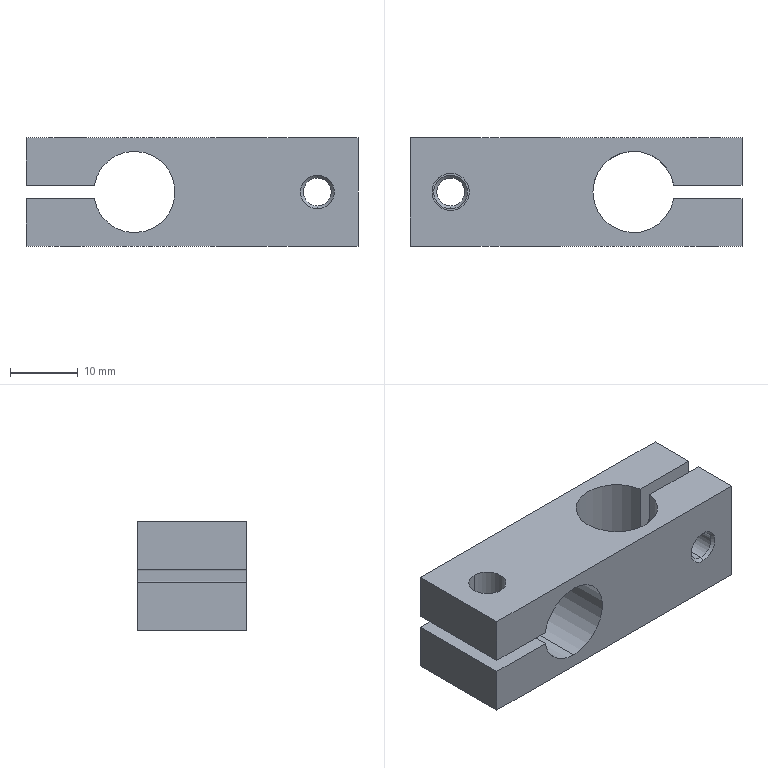Part | STEP file | 11-KDST12_b-ab11 | 1 solid | 33 faces | box 49 x 16 x 16 mm | volume 7757 mm3 | cylinder 13 | plane 12 | cone 8 | commonest cylinder face diameters 12 x5 4.134 x4 5.5 x4
STEP:
#1=CARTESIAN_POINT('',(-27.,2.75,1.));
#2=VERTEX_POINT('',#1);
#3=CARTESIAN_POINT('',(-27.,-2.75,1.));
#4=VERTEX_POINT('',#3);
#5=CARTESIAN_POINT('',(-27.,0.,1.));
#6=DIRECTION('',(0.,0.,1.));
#7=DIRECTION('',(-1.,0.,0.));
#8=AXIS2_PLACEMENT_3D('',#5,#6,#7);
#9=CIRCLE('',#8,2.75);
#10=EDGE_CURVE('',#2,#4,#9,.T.);
#11=ORIENTED_EDGE('',*,*,#10,.F.);
#12=CARTESIAN_POINT('',(-27.,2.75,8.));
#13=VERTEX_POINT('',#12);
#14=CARTESIAN_POINT('',(-27.,2.75,-8.));
#15=DIRECTION('',(0.,0.,1.));
#16=VECTOR('',#15,1000.);
#17=LINE('',#14,#16);
#18=EDGE_CURVE('',#2,#13,#17,.T.);
#19=ORIENTED_EDGE('',*,*,#18,.T.);
#20=CARTESIAN_POINT('',(-27.,-2.75,8.));
#21=VERTEX_POINT('',#20);
#22=CARTESIAN_POINT('',(-27.,0.,8.));
#23=DIRECTION('',(0.,0.,1.));
#24=DIRECTION('',(0.,-1.,0.));
#25=AXIS2_PLACEMENT_3D('',#22,#23,#24);
#26=CIRCLE('',#25,2.75);
#27=EDGE_CURVE('',#13,#21,#26,.T.);
#28=ORIENTED_EDGE('',*,*,#27,.T.);
#29=CARTESIAN_POINT('',(-27.,-2.75,-8.));
#30=DIRECTION('',(0.,0.,1.));
#31=VECTOR('',#30,1000.);
#32=LINE('',#29,#31);
#33=EDGE_CURVE('',#4,#21,#32,.T.);
#34=ORIENTED_EDGE('',*,*,#33,.F.);
#35=EDGE_LOOP('',(#11,#19,#28,#34));
#36=FACE_OUTER_BOUND('',#35,.T.);
#37=CARTESIAN_POINT('',(-27.,0.,-8.));
#38=DIRECTION('',(0.,0.,1.));
#39=DIRECTION('',(0.,-1.,0.));
#40=AXIS2_PLACEMENT_3D('',#37,#38,#39);
#41=CYLINDRICAL_SURFACE('',#40,2.75);
#42=ADVANCED_FACE('',(#36),#41,.F.);
#43=CARTESIAN_POINT('',(-27.,2.067,-1.433));
#44=VERTEX_POINT('',#43);
#45=CARTESIAN_POINT('',(-27.,-2.067,-1.433));
#46=VERTEX_POINT('',#45);
#47=CARTESIAN_POINT('',(-27.,0.,-1.433));
#48=DIRECTION('',(0.,0.,1.));
#49=DIRECTION('',(0.,-1.,0.));
#50=AXIS2_PLACEMENT_3D('',#47,#48,#49);
#51=CIRCLE('',#50,2.067);
#52=EDGE_CURVE('',#44,#46,#51,.T.);
#53=ORIENTED_EDGE('',*,*,#52,.F.);
#54=CARTESIAN_POINT('',(-27.,2.5,-1.));
#55=VERTEX_POINT('',#54);
#56=CARTESIAN_POINT('',(-27.,2.067,-1.433));
#57=DIRECTION('',(0.,0.7071,0.7071));
#58=VECTOR('',#57,1000.);
#59=LINE('',#56,#58);
#60=EDGE_CURVE('',#44,#55,#59,.T.);
#61=ORIENTED_EDGE('',*,*,#60,.T.);
#62=CARTESIAN_POINT('',(-27.,-2.5,-1.));
#63=VERTEX_POINT('',#62);
#64=CARTESIAN_POINT('',(-27.,0.,-1.));
#65=DIRECTION('',(0.,0.,1.));
#66=DIRECTION('',(0.,-1.,0.));
#67=AXIS2_PLACEMENT_3D('',#64,#65,#66);
#68=CIRCLE('',#67,2.5);
#69=EDGE_CURVE('',#55,#63,#68,.T.);
#70=ORIENTED_EDGE('',*,*,#69,.T.);
#71=CARTESIAN_POINT('',(-27.,-2.067,-1.433));
#72=DIRECTION('',(0.,-0.7071,0.7071));
#73=VECTOR('',#72,1000.);
#74=LINE('',#71,#73);
#75=EDGE_CURVE('',#46,#63,#74,.T.);
#76=ORIENTED_EDGE('',*,*,#75,.F.);
#77=EDGE_LOOP('',(#53,#61,#70,#76));
#78=FACE_OUTER_BOUND('',#77,.T.);
#79=CARTESIAN_POINT('',(-27.,0.,-1.433));
#80=DIRECTION('',(0.,0.,1.));
#81=DIRECTION('',(0.,-1.,0.));
#82=AXIS2_PLACEMENT_3D('',#79,#80,#81);
#83=CONICAL_SURFACE('',#82,2.067,0.7854);
#84=ADVANCED_FACE('',(#78),#83,.F.);
#85=CARTESIAN_POINT('',(-27.,2.067,-7.567));
#86=VERTEX_POINT('',#85);
#87=CARTESIAN_POINT('',(-27.,-2.067,-7.567));
#88=VERTEX_POINT('',#87);
#89=CARTESIAN_POINT('',(-27.,0.,-7.567));
#90=DIRECTION('',(0.,0.,1.));
#91=DIRECTION('',(0.,-1.,0.));
#92=AXIS2_PLACEMENT_3D('',#89,#90,#91);
#93=CIRCLE('',#92,2.067);
#94=EDGE_CURVE('',#86,#88,#93,.T.);
#95=ORIENTED_EDGE('',*,*,#94,.F.);
#96=CARTESIAN_POINT('',(-27.,2.067,-8.));
#97=DIRECTION('',(0.,0.,1.));
#98=VECTOR('',#97,1000.);
#99=LINE('',#96,#98);
#100=EDGE_CURVE('',#86,#44,#99,.T.);
#101=ORIENTED_EDGE('',*,*,#100,.T.);
#102=ORIENTED_EDGE('',*,*,#52,.T.);
#103=CARTESIAN_POINT('',(-27.,-2.067,-8.));
#104=DIRECTION('',(0.,0.,1.));
#105=VECTOR('',#104,1000.);
#106=LINE('',#103,#105);
#107=EDGE_CURVE('',#88,#46,#106,.T.);
#108=ORIENTED_EDGE('',*,*,#107,.F.);
#109=EDGE_LOOP('',(#95,#101,#102,#108));
#110=FACE_OUTER_BOUND('',#109,.T.);
#111=CARTESIAN_POINT('',(-27.,0.,-8.));
#112=DIRECTION('',(0.,0.,1.));
#113=DIRECTION('',(0.,-1.,0.));
#114=AXIS2_PLACEMENT_3D('',#111,#112,#113);
#115=CYLINDRICAL_SURFACE('',#114,2.067);
#116=ADVANCED_FACE('',(#110),#115,.F.);
#117=ORIENTED_EDGE('',*,*,#94,.T.);
#118=CARTESIAN_POINT('',(-27.,-2.5,-8.));
#119=VERTEX_POINT('',#118);
#120=CARTESIAN_POINT('',(-27.,-2.5,-8.));
#121=DIRECTION('',(0.,-0.7071,-0.7071));
#122=VECTOR('',#121,1000.);
#123=LINE('',#120,#122);
#124=EDGE_CURVE('',#88,#119,#123,.T.);
#125=ORIENTED_EDGE('',*,*,#124,.T.);
#126=CARTESIAN_POINT('',(-27.,2.5,-8.));
#127=VERTEX_POINT('',#126);
#128=CARTESIAN_POINT('',(-27.,0.,-8.));
#129=DIRECTION('',(0.,0.,1.));
#130=DIRECTION('',(0.,-1.,0.));
#131=AXIS2_PLACEMENT_3D('',#128,#129,#130);
#132=CIRCLE('',#131,2.5);
#133=EDGE_CURVE('',#127,#119,#132,.T.);
#134=ORIENTED_EDGE('',*,*,#133,.F.);
#135=CARTESIAN_POINT('',(-27.,2.5,-8.));
#136=DIRECTION('',(0.,0.7071,-0.7071));
#137=VECTOR('',#136,1000.);
#138=LINE('',#135,#137);
#139=EDGE_CURVE('',#86,#127,#138,.T.);
#140=ORIENTED_EDGE('',*,*,#139,.F.);
#141=EDGE_LOOP('',(#117,#125,#134,#140));
#142=FACE_OUTER_BOUND('',#141,.T.);
#143=CARTESIAN_POINT('',(-27.,0.,-8.));
#144=DIRECTION('',(0.,0.,-1.));
#145=DIRECTION('',(0.,1.,0.));
#146=AXIS2_PLACEMENT_3D('',#143,#144,#145);
#147=CONICAL_SURFACE('',#146,2.5,0.7854);
#148=ADVANCED_FACE('',(#142),#147,.F.);
#149=CARTESIAN_POINT('',(10.,-7.567,-2.067));
#150=VERTEX_POINT('',#149);
#151=CARTESIAN_POINT('',(10.,-7.567,2.067));
#152=VERTEX_POINT('',#151);
#153=CARTESIAN_POINT('',(10.,-7.567,0.));
#154=DIRECTION('',(0.,1.,0.));
#155=DIRECTION('',(0.,0.,1.));
#156=AXIS2_PLACEMENT_3D('',#153,#154,#155);
#157=CIRCLE('',#156,2.067);
#158=EDGE_CURVE('',#150,#152,#157,.T.);
#159=ORIENTED_EDGE('',*,*,#158,.T.);
#160=CARTESIAN_POINT('',(10.,-8.,2.5));
#161=VERTEX_POINT('',#160);
#162=CARTESIAN_POINT('',(10.,-8.,2.5));
#163=DIRECTION('',(0.,-0.7071,0.7071));
#164=VECTOR('',#163,1000.);
#165=LINE('',#162,#164);
#166=EDGE_CURVE('',#152,#161,#165,.T.);
#167=ORIENTED_EDGE('',*,*,#166,.T.);
#168=CARTESIAN_POINT('',(10.,-8.,-2.5));
#169=VERTEX_POINT('',#168);
#170=CARTESIAN_POINT('',(10.,-8.,0.));
#171=DIRECTION('',(0.,1.,0.));
#172=DIRECTION('',(0.,0.,1.));
#173=AXIS2_PLACEMENT_3D('',#170,#171,#172);
#174=CIRCLE('',#173,2.5);
#175=EDGE_CURVE('',#169,#161,#174,.T.);
#176=ORIENTED_EDGE('',*,*,#175,.F.);
#177=CARTESIAN_POINT('',(10.,-8.,-2.5));
#178=DIRECTION('',(0.,-0.7071,-0.7071));
#179=VECTOR('',#178,1000.);
#180=LINE('',#177,#179);
#181=EDGE_CURVE('',#150,#169,#180,.T.);
#182=ORIENTED_EDGE('',*,*,#181,.F.);
#183=EDGE_LOOP('',(#159,#167,#176,#182));
#184=FACE_OUTER_BOUND('',#183,.T.);
#185=CARTESIAN_POINT('',(10.,-8.,0.));
#186=DIRECTION('',(0.,-1.,0.));
#187=DIRECTION('',(0.,0.,-1.));
#188=AXIS2_PLACEMENT_3D('',#185,#186,#187);
#189=CONICAL_SURFACE('',#188,2.5,0.7854);
#190=ADVANCED_FACE('',(#184),#189,.F.);
#191=ORIENTED_EDGE('',*,*,#158,.F.);
#192=CARTESIAN_POINT('',(10.,-1.433,-2.067));
#193=VERTEX_POINT('',#192);
#194=CARTESIAN_POINT('',(10.,-8.,-2.067));
#195=DIRECTION('',(0.,1.,0.));
#196=VECTOR('',#195,1000.);
#197=LINE('',#194,#196);
#198=EDGE_CURVE('',#150,#193,#197,.T.);
#199=ORIENTED_EDGE('',*,*,#198,.T.);
#200=CARTESIAN_POINT('',(10.,-1.433,2.067));
#201=VERTEX_POINT('',#200);
#202=CARTESIAN_POINT('',(10.,-1.433,0.));
#203=DIRECTION('',(0.,1.,0.));
#204=DIRECTION('',(0.,0.,1.));
#205=AXIS2_PLACEMENT_3D('',#202,#203,#204);
#206=CIRCLE('',#205,2.067);
#207=EDGE_CURVE('',#193,#201,#206,.T.);
#208=ORIENTED_EDGE('',*,*,#207,.T.);
#209=CARTESIAN_POINT('',(10.,-8.,2.067));
#210=DIRECTION('',(0.,1.,0.));
#211=VECTOR('',#210,1000.);
#212=LINE('',#209,#211);
#213=EDGE_CURVE('',#152,#201,#212,.T.);
#214=ORIENTED_EDGE('',*,*,#213,.F.);
#215=EDGE_LOOP('',(#191,#199,#208,#214));
#216=FACE_OUTER_BOUND('',#215,.T.);
#217=CARTESIAN_POINT('',(10.,-8.,0.));
#218=DIRECTION('',(0.,1.,0.));
#219=DIRECTION('',(0.,0.,1.));
#220=AXIS2_PLACEMENT_3D('',#217,#218,#219);
#221=CYLINDRICAL_SURFACE('',#220,2.067);
#222=ADVANCED_FACE('',(#216),#221,.F.);
#223=ORIENTED_EDGE('',*,*,#207,.F.);
#224=CARTESIAN_POINT('',(10.,-1.,-2.5));
#225=VERTEX_POINT('',#224);
#226=CARTESIAN_POINT('',(10.,-1.433,-2.067));
#227=DIRECTION('',(0.,0.7071,-0.7071));
#228=VECTOR('',#227,1000.);
#229=LINE('',#226,#228);
#230=EDGE_CURVE('',#193,#225,#229,.T.);
#231=ORIENTED_EDGE('',*,*,#230,.T.);
#232=CARTESIAN_POINT('',(10.,-1.,2.5));
#233=VERTEX_POINT('',#232);
#234=CARTESIAN_POINT('',(10.,-1.,0.));
#235=DIRECTION('',(0.,1.,0.));
#236=DIRECTION('',(0.,0.,1.));
#237=AXIS2_PLACEMENT_3D('',#234,#235,#236);
#238=CIRCLE('',#237,2.5);
#239=EDGE_CURVE('',#225,#233,#238,.T.);
#240=ORIENTED_EDGE('',*,*,#239,.T.);
#241=CARTESIAN_POINT('',(10.,-1.433,2.067));
#242=DIRECTION('',(0.,0.7071,0.7071));
#243=VECTOR('',#242,1000.);
#244=LINE('',#241,#243);
#245=EDGE_CURVE('',#201,#233,#244,.T.);
#246=ORIENTED_EDGE('',*,*,#245,.F.);
#247=EDGE_LOOP('',(#223,#231,#240,#246));
#248=FACE_OUTER_BOUND('',#247,.T.);
#249=CARTESIAN_POINT('',(10.,-1.433,0.));
#250=DIRECTION('',(0.,1.,0.));
#251=DIRECTION('',(0.,0.,1.));
#252=AXIS2_PLACEMENT_3D('',#249,#250,#251);
#253=CONICAL_SURFACE('',#252,2.067,0.7854);
#254=ADVANCED_FACE('',(#248),#253,.F.);
#255=CARTESIAN_POINT('',(10.,1.,2.75));
#256=VERTEX_POINT('',#255);
#257=CARTESIAN_POINT('',(10.,1.,-2.75));
#258=VERTEX_POINT('',#257);
#259=CARTESIAN_POINT('',(10.,1.,0.));
#260=DIRECTION('',(0.,-1.,0.));
#261=DIRECTION('',(0.,0.,1.));
#262=AXIS2_PLACEMENT_3D('',#259,#260,#261);
#263=CIRCLE('',#262,2.75);
#264=EDGE_CURVE('',#256,#258,#263,.T.);
#265=ORIENTED_EDGE('',*,*,#264,.T.);
#266=CARTESIAN_POINT('',(10.,8.,-2.75));
#267=VERTEX_POINT('',#266);
#268=CARTESIAN_POINT('',(10.,-8.,-2.75));
#269=DIRECTION('',(0.,1.,0.));
#270=VECTOR('',#269,1000.);
#271=LINE('',#268,#270);
#272=EDGE_CURVE('',#258,#267,#271,.T.);
#273=ORIENTED_EDGE('',*,*,#272,.T.);
#274=CARTESIAN_POINT('',(10.,8.,2.75));
#275=VERTEX_POINT('',#274);
#276=CARTESIAN_POINT('',(10.,8.,0.));
#277=DIRECTION('',(0.,1.,0.));
#278=DIRECTION('',(0.,0.,1.));
#279=AXIS2_PLACEMENT_3D('',#276,#277,#278);
#280=CIRCLE('',#279,2.75);
#281=EDGE_CURVE('',#267,#275,#280,.T.);
#282=ORIENTED_EDGE('',*,*,#281,.T.);
#283=CARTESIAN_POINT('',(10.,-8.,2.75));
#284=DIRECTION('',(0.,1.,0.));
#285=VECTOR('',#284,1000.);
#286=LINE('',#283,#285);
#287=EDGE_CURVE('',#256,#275,#286,.T.);
#288=ORIENTED_EDGE('',*,*,#287,.F.);
#289=EDGE_LOOP('',(#265,#273,#282,#288));
#290=FACE_OUTER_BOUND('',#289,.T.);
#291=CARTESIAN_POINT('',(10.,-8.,0.));
#292=DIRECTION('',(0.,1.,0.));
#293=DIRECTION('',(0.,0.,1.));
#294=AXIS2_PLACEMENT_3D('',#291,#292,#293);
#295=CYLINDRICAL_SURFACE('',#294,2.75);
#296=ADVANCED_FACE('',(#290),#295,.F.);
#297=CARTESIAN_POINT('',(-22.916,-8.,-1.));
#298=VERTEX_POINT('',#297);
#299=CARTESIAN_POINT('',(-17.,-8.,-6.));
#300=VERTEX_POINT('',#299);
#301=CARTESIAN_POINT('',(-17.,-8.,0.));
#302=DIRECTION('',(0.,-1.,0.));
#303=DIRECTION('',(0.,0.,-1.));
#304=AXIS2_PLACEMENT_3D('',#301,#302,#303);
#305=CIRCLE('',#304,6.);
#306=EDGE_CURVE('',#298,#300,#305,.T.);
#307=ORIENTED_EDGE('',*,*,#306,.T.);
#308=CARTESIAN_POINT('',(-17.,8.,-6.));
#309=VERTEX_POINT('',#308);
#310=CARTESIAN_POINT('',(-17.,-8.,-6.));
#311=DIRECTION('',(0.,1.,0.));
#312=VECTOR('',#311,1000.);
#313=LINE('',#310,#312);
#314=EDGE_CURVE('',#300,#309,#313,.T.);
#315=ORIENTED_EDGE('',*,*,#314,.T.);
#316=CARTESIAN_POINT('',(-22.916,8.,-1.));
#317=VERTEX_POINT('',#316);
#318=CARTESIAN_POINT('',(-17.,8.,0.));
#319=DIRECTION('',(0.,-1.,0.));
#320=DIRECTION('',(0.,0.,-1.));
#321=AXIS2_PLACEMENT_3D('',#318,#319,#320);
#322=CIRCLE('',#321,6.);
#323=EDGE_CURVE('',#317,#309,#322,.T.);
#324=ORIENTED_EDGE('',*,*,#323,.F.);
#325=CARTESIAN_POINT('',(-22.916,-8.,-1.));
#326=DIRECTION('',(0.,1.,0.));
#327=VECTOR('',#326,1000.);
#328=LINE('',#325,#327);
#329=EDGE_CURVE('',#298,#317,#328,.T.);
#330=ORIENTED_EDGE('',*,*,#329,.F.);
#331=EDGE_LOOP('',(#307,#315,#324,#330));
#332=FACE_OUTER_BOUND('',#331,.T.);
#333=CARTESIAN_POINT('',(-17.,-8.,0.));
#334=DIRECTION('',(0.,1.,0.));
#335=DIRECTION('',(0.,0.,1.));
#336=AXIS2_PLACEMENT_3D('',#333,#334,#335);
#337=CYLINDRICAL_SURFACE('',#336,6.);
#338=ADVANCED_FACE('',(#332),#337,.F.);
#339=ORIENTED_EDGE('',*,*,#314,.F.);
#340=CARTESIAN_POINT('',(-17.,-8.,6.));
#341=VERTEX_POINT('',#340);
#342=CARTESIAN_POINT('',(-17.,-8.,0.));
#343=DIRECTION('',(0.,-1.,0.));
#344=DIRECTION('',(0.,0.,-1.));
#345=AXIS2_PLACEMENT_3D('',#342,#343,#344);
#346=CIRCLE('',#345,6.);
#347=EDGE_CURVE('',#300,#341,#346,.T.);
#348=ORIENTED_EDGE('',*,*,#347,.T.);
#349=CARTESIAN_POINT('',(-17.,8.,6.));
#350=VERTEX_POINT('',#349);
#351=CARTESIAN_POINT('',(-17.,-8.,6.));
#352=DIRECTION('',(0.,1.,0.));
#353=VECTOR('',#352,1000.);
#354=LINE('',#351,#353);
#355=EDGE_CURVE('',#341,#350,#354,.T.);
#356=ORIENTED_EDGE('',*,*,#355,.T.);
#357=CARTESIAN_POINT('',(-17.,8.,0.));
#358=DIRECTION('',(0.,-1.,0.));
#359=DIRECTION('',(0.,0.,-1.));
#360=AXIS2_PLACEMENT_3D('',#357,#358,#359);
#361=CIRCLE('',#360,6.);
#362=EDGE_CURVE('',#309,#350,#361,.T.);
#363=ORIENTED_EDGE('',*,*,#362,.F.);
#364=EDGE_LOOP('',(#339,#348,#356,#363));
#365=FACE_OUTER_BOUND('',#364,.T.);
#366=CARTESIAN_POINT('',(-17.,-8.,0.));
#367=DIRECTION('',(0.,1.,0.));
#368=DIRECTION('',(0.,0.,1.));
#369=AXIS2_PLACEMENT_3D('',#366,#367,#368);
#370=CYLINDRICAL_SURFACE('',#369,6.);
#371=ADVANCED_FACE('',(#365),#370,.F.);
#372=CARTESIAN_POINT('',(-6.,0.,8.));
#373=VERTEX_POINT('',#372);
#374=CARTESIAN_POINT('',(5.916,1.,8.));
#375=VERTEX_POINT('',#374);
#376=CARTESIAN_POINT('',(0.,0.,8.));
#377=DIRECTION('',(0.,0.,-1.));
#378=DIRECTION('',(-1.,0.,0.));
#379=AXIS2_PLACEMENT_3D('',#376,#377,#378);
#380=CIRCLE('',#379,6.);
#381=EDGE_CURVE('',#373,#375,#380,.T.);
#382=ORIENTED_EDGE('',*,*,#381,.F.);
#383=CARTESIAN_POINT('',(-6.,0.,-8.));
#384=VERTEX_POINT('',#383);
#385=CARTESIAN_POINT('',(-6.,0.,8.));
#386=DIRECTION('',(0.,0.,-1.));
#387=VECTOR('',#386,1000.);
#388=LINE('',#385,#387);
#389=EDGE_CURVE('',#373,#384,#388,.T.);
#390=ORIENTED_EDGE('',*,*,#389,.T.);
#391=CARTESIAN_POINT('',(5.916,1.,-8.));
#392=VERTEX_POINT('',#391);
#393=CARTESIAN_POINT('',(0.,0.,-8.));
#394=DIRECTION('',(0.,0.,-1.));
#395=DIRECTION('',(-1.,0.,0.));
#396=AXIS2_PLACEMENT_3D('',#393,#394,#395);
#397=CIRCLE('',#396,6.);
#398=EDGE_CURVE('',#384,#392,#397,.T.);
#399=ORIENTED_EDGE('',*,*,#398,.T.);
#400=CARTESIAN_POINT('',(5.916,1.,8.));
#401=DIRECTION('',(0.,0.,-1.));
#402=VECTOR('',#401,1000.);
#403=LINE('',#400,#402);
#404=EDGE_CURVE('',#375,#392,#403,.T.);
#405=ORIENTED_EDGE('',*,*,#404,.F.);
#406=EDGE_LOOP('',(#382,#390,#399,#405));
#407=FACE_OUTER_BOUND('',#406,.T.);
#408=CARTESIAN_POINT('',(0.,0.,8.));
#409=DIRECTION('',(0.,0.,-1.));
#410=DIRECTION('',(-1.,0.,0.));
#411=AXIS2_PLACEMENT_3D('',#408,#409,#410);
#412=CYLINDRICAL_SURFACE('',#411,6.);
#413=ADVANCED_FACE('',(#407),#412,.F.);
#414=CARTESIAN_POINT('',(10.,8.,0.));
#415=DIRECTION('',(0.,1.,0.));
#416=DIRECTION('',(0.,0.,1.));
#417=AXIS2_PLACEMENT_3D('',#414,#415,#416);
#418=CIRCLE('',#417,2.75);
#419=EDGE_CURVE('',#275,#267,#418,.T.);
#420=ORIENTED_EDGE('',*,*,#419,.F.);
#421=ORIENTED_EDGE('',*,*,#281,.F.);
#422=EDGE_LOOP('',(#420,#421));
#423=FACE_BOUND('',#422,.T.);
#424=CARTESIAN_POINT('',(-22.916,8.,1.));
#425=VERTEX_POINT('',#424);
#426=CARTESIAN_POINT('',(-33.,8.,1.));
#427=VERTEX_POINT('',#426);
#428=CARTESIAN_POINT('',(-22.916,8.,1.));
#429=DIRECTION('',(-1.,0.,0.));
#430=VECTOR('',#429,1000.);
#431=LINE('',#428,#430);
#432=EDGE_CURVE('',#425,#427,#431,.T.);
#433=ORIENTED_EDGE('',*,*,#432,.T.);
#434=CARTESIAN_POINT('',(-33.,8.,8.));
#435=VERTEX_POINT('',#434);
#436=CARTESIAN_POINT('',(-33.,8.,8.));
#437=DIRECTION('',(0.,0.,-1.));
#438=VECTOR('',#437,1000.);
#439=LINE('',#436,#438);
#440=EDGE_CURVE('',#435,#427,#439,.T.);
#441=ORIENTED_EDGE('',*,*,#440,.F.);
#442=CARTESIAN_POINT('',(16.,8.,8.));
#443=VERTEX_POINT('',#442);
#444=CARTESIAN_POINT('',(16.,8.,8.));
#445=DIRECTION('',(-1.,0.,0.));
#446=VECTOR('',#445,1000.);
#447=LINE('',#444,#446);
#448=EDGE_CURVE('',#443,#435,#447,.T.);
#449=ORIENTED_EDGE('',*,*,#448,.F.);
#450=CARTESIAN_POINT('',(16.,8.,-8.));
#451=VERTEX_POINT('',#450);
#452=CARTESIAN_POINT('',(16.,8.,8.));
#453=DIRECTION('',(0.,0.,-1.));
#454=VECTOR('',#453,1000.);
#455=LINE('',#452,#454);
#456=EDGE_CURVE('',#443,#451,#455,.T.);
#457=ORIENTED_EDGE('',*,*,#456,.T.);
#458=CARTESIAN_POINT('',(-33.,8.,-8.));
#459=VERTEX_POINT('',#458);
#460=CARTESIAN_POINT('',(16.,8.,-8.));
#461=DIRECTION('',(-1.,0.,0.));
#462=VECTOR('',#461,1000.);
#463=LINE('',#460,#462);
#464=EDGE_CURVE('',#451,#459,#463,.T.);
#465=ORIENTED_EDGE('',*,*,#464,.T.);
#466=CARTESIAN_POINT('',(-33.,8.,-1.));
#467=VERTEX_POINT('',#466);
#468=CARTESIAN_POINT('',(-33.,8.,8.));
#469=DIRECTION('',(0.,0.,-1.));
#470=VECTOR('',#469,1000.);
#471=LINE('',#468,#470);
#472=EDGE_CURVE('',#467,#459,#471,.T.);
#473=ORIENTED_EDGE('',*,*,#472,.F.);
#474=CARTESIAN_POINT('',(-33.,8.,-1.));
#475=DIRECTION('',(1.,0.,0.));
#476=VECTOR('',#475,1000.);
#477=LINE('',#474,#476);
#478=EDGE_CURVE('',#467,#317,#477,.T.);
#479=ORIENTED_EDGE('',*,*,#478,.T.);
#480=ORIENTED_EDGE('',*,*,#323,.T.);
#481=ORIENTED_EDGE('',*,*,#362,.T.);
#482=CARTESIAN_POINT('',(-17.,8.,0.));
#483=DIRECTION('',(0.,-1.,0.));
#484=DIRECTION('',(0.,0.,-1.));
#485=AXIS2_PLACEMENT_3D('',#482,#483,#484);
#486=CIRCLE('',#485,6.);
#487=EDGE_CURVE('',#350,#425,#486,.T.);
#488=ORIENTED_EDGE('',*,*,#487,.T.);
#489=EDGE_LOOP('',(#433,#441,#449,#457,#465,#473,#479,#480,#481,#488));
#490=FACE_OUTER_BOUND('',#489,.T.);
#491=CARTESIAN_POINT('',(16.,8.,8.));
#492=DIRECTION('',(0.,-1.,0.));
#493=DIRECTION('',(0.,0.,-1.));
#494=AXIS2_PLACEMENT_3D('',#491,#492,#493);
#495=PLANE('',#494);
#496=ADVANCED_FACE('',(#423,#490),#495,.F.);
#497=CARTESIAN_POINT('',(-33.,-8.,1.));
#498=VERTEX_POINT('',#497);
#499=CARTESIAN_POINT('',(-33.,-8.,1.));
#500=DIRECTION('',(0.,1.,0.));
#501=VECTOR('',#500,1000.);
#502=LINE('',#499,#501);
#503=EDGE_CURVE('',#498,#427,#502,.T.);
#504=ORIENTED_EDGE('',*,*,#503,.F.);
#505=CARTESIAN_POINT('',(-33.,-8.,8.));
#506=VERTEX_POINT('',#505);
#507=CARTESIAN_POINT('',(-33.,-8.,8.));
#508=DIRECTION('',(0.,0.,-1.));
#509=VECTOR('',#508,1000.);
#510=LINE('',#507,#509);
#511=EDGE_CURVE('',#506,#498,#510,.T.);
#512=ORIENTED_EDGE('',*,*,#511,.F.);
#513=CARTESIAN_POINT('',(-33.,8.,8.));
#514=DIRECTION('',(0.,-1.,0.));
#515=VECTOR('',#514,1000.);
#516=LINE('',#513,#515);
#517=EDGE_CURVE('',#435,#506,#516,.T.);
#518=ORIENTED_EDGE('',*,*,#517,.F.);
#519=ORIENTED_EDGE('',*,*,#440,.T.);
#520=EDGE_LOOP('',(#504,#512,#518,#519));
#521=FACE_OUTER_BOUND('',#520,.T.);
#522=CARTESIAN_POINT('',(-33.,8.,8.));
#523=DIRECTION('',(1.,0.,0.));
#524=DIRECTION('',(0.,0.,-1.));
#525=AXIS2_PLACEMENT_3D('',#522,#523,#524);
#526=PLANE('',#525);
#527=ADVANCED_FACE('',(#521),#526,.F.);
#528=CARTESIAN_POINT('',(-33.,-8.,-1.));
#529=VERTEX_POINT('',#528);
#530=CARTESIAN_POINT('',(-33.,-8.,-1.));
#531=DIRECTION('',(0.,1.,0.));
#532=VECTOR('',#531,1000.);
#533=LINE('',#530,#532);
#534=EDGE_CURVE('',#529,#467,#533,.T.);
#535=ORIENTED_EDGE('',*,*,#534,.T.);
#536=ORIENTED_EDGE('',*,*,#472,.T.);
#537=CARTESIAN_POINT('',(-33.,-8.,-8.));
#538=VERTEX_POINT('',#537);
#539=CARTESIAN_POINT('',(-33.,8.,-8.));
#540=DIRECTION('',(0.,-1.,0.));
#541=VECTOR('',#540,1000.);
#542=LINE('',#539,#541);
#543=EDGE_CURVE('',#459,#538,#542,.T.);
#544=ORIENTED_EDGE('',*,*,#543,.T.);
#545=CARTESIAN_POINT('',(-33.,-8.,8.));
#546=DIRECTION('',(0.,0.,-1.));
#547=VECTOR('',#546,1000.);
#548=LINE('',#545,#547);
#549=EDGE_CURVE('',#529,#538,#548,.T.);
#550=ORIENTED_EDGE('',*,*,#549,.F.);
#551=EDGE_LOOP('',(#535,#536,#544,#550));
#552=FACE_OUTER_BOUND('',#551,.T.);
#553=CARTESIAN_POINT('',(-33.,8.,8.));
#554=DIRECTION('',(1.,0.,0.));
#555=DIRECTION('',(0.,0.,-1.));
#556=AXIS2_PLACEMENT_3D('',#553,#554,#555);
#557=PLANE('',#556);
#558=ADVANCED_FACE('',(#552),#557,.F.);
#559=ORIENTED_EDGE('',*,*,#175,.T.);
#560=CARTESIAN_POINT('',(10.,-8.,0.));
#561=DIRECTION('',(0.,1.,0.));
#562=DIRECTION('',(0.,0.,1.));
#563=AXIS2_PLACEMENT_3D('',#560,#561,#562);
#564=CIRCLE('',#563,2.5);
#565=EDGE_CURVE('',#161,#169,#564,.T.);
#566=ORIENTED_EDGE('',*,*,#565,.T.);
#567=EDGE_LOOP('',(#559,#566));
#568=FACE_BOUND('',#567,.T.);
#569=CARTESIAN_POINT('',(-22.916,-8.,1.));
#570=VERTEX_POINT('',#569);
#571=CARTESIAN_POINT('',(-22.916,-8.,1.));
#572=DIRECTION('',(-1.,0.,0.));
#573=VECTOR('',#572,1000.);
#574=LINE('',#571,#573);
#575=EDGE_CURVE('',#570,#498,#574,.T.);
#576=ORIENTED_EDGE('',*,*,#575,.F.);
#577=CARTESIAN_POINT('',(-17.,-8.,0.));
#578=DIRECTION('',(0.,-1.,0.));
#579=DIRECTION('',(0.,0.,-1.));
#580=AXIS2_PLACEMENT_3D('',#577,#578,#579);
#581=CIRCLE('',#580,6.);
#582=EDGE_CURVE('',#341,#570,#581,.T.);
#583=ORIENTED_EDGE('',*,*,#582,.F.);
#584=ORIENTED_EDGE('',*,*,#347,.F.);
#585=ORIENTED_EDGE('',*,*,#306,.F.);
#586=CARTESIAN_POINT('',(-33.,-8.,-1.));
#587=DIRECTION('',(1.,0.,0.));
#588=VECTOR('',#587,1000.);
#589=LINE('',#586,#588);
#590=EDGE_CURVE('',#529,#298,#589,.T.);
#591=ORIENTED_EDGE('',*,*,#590,.F.);
#592=ORIENTED_EDGE('',*,*,#549,.T.);
#593=CARTESIAN_POINT('',(16.,-8.,-8.));
#594=VERTEX_POINT('',#593);
#595=CARTESIAN_POINT('',(-33.,-8.,-8.));
#596=DIRECTION('',(1.,0.,0.));
#597=VECTOR('',#596,1000.);
#598=LINE('',#595,#597);
#599=EDGE_CURVE('',#538,#594,#598,.T.);
#600=ORIENTED_EDGE('',*,*,#599,.T.);
#601=CARTESIAN_POINT('',(16.,-8.,8.));
#602=VERTEX_POINT('',#601);
#603=CARTESIAN_POINT('',(16.,-8.,8.));
#604=DIRECTION('',(0.,0.,-1.));
#605=VECTOR('',#604,1000.);
#606=LINE('',#603,#605);
#607=EDGE_CURVE('',#602,#594,#606,.T.);
#608=ORIENTED_EDGE('',*,*,#607,.F.);
#609=CARTESIAN_POINT('',(-33.,-8.,8.));
#610=DIRECTION('',(1.,0.,0.));
#611=VECTOR('',#610,1000.);
#612=LINE('',#609,#611);
#613=EDGE_CURVE('',#506,#602,#612,.T.);
#614=ORIENTED_EDGE('',*,*,#613,.F.);
#615=ORIENTED_EDGE('',*,*,#511,.T.);
#616=EDGE_LOOP('',(#576,#583,#584,#585,#591,#592,#600,#608,#614,#615));
#617=FACE_OUTER_BOUND('',#616,.T.);
#618=CARTESIAN_POINT('',(-33.,-8.,8.));
#619=DIRECTION('',(0.,1.,0.));
#620=DIRECTION('',(0.,0.,1.));
#621=AXIS2_PLACEMENT_3D('',#618,#619,#620);
#622=PLANE('',#621);
#623=ADVANCED_FACE('',(#568,#617),#622,.F.);
#624=ORIENTED_EDGE('',*,*,#607,.T.);
#625=CARTESIAN_POINT('',(16.,-1.,-8.));
#626=VERTEX_POINT('',#625);
#627=CARTESIAN_POINT('',(16.,-8.,-8.));
#628=DIRECTION('',(0.,1.,0.));
#629=VECTOR('',#628,1000.);
#630=LINE('',#627,#629);
#631=EDGE_CURVE('',#594,#626,#630,.T.);
#632=ORIENTED_EDGE('',*,*,#631,.T.);
#633=CARTESIAN_POINT('',(16.,-1.,8.));
#634=VERTEX_POINT('',#633);
#635=CARTESIAN_POINT('',(16.,-1.,8.));
#636=DIRECTION('',(0.,0.,-1.));
#637=VECTOR('',#636,1000.);
#638=LINE('',#635,#637);
#639=EDGE_CURVE('',#634,#626,#638,.T.);
#640=ORIENTED_EDGE('',*,*,#639,.F.);
#641=CARTESIAN_POINT('',(16.,-8.,8.));
#642=DIRECTION('',(0.,1.,0.));
#643=VECTOR('',#642,1000.);
#644=LINE('',#641,#643);
#645=EDGE_CURVE('',#602,#634,#644,.T.);
#646=ORIENTED_EDGE('',*,*,#645,.F.);
#647=EDGE_LOOP('',(#624,#632,#640,#646));
#648=FACE_OUTER_BOUND('',#647,.T.);
#649=CARTESIAN_POINT('',(16.,-8.,8.));
#650=DIRECTION('',(-1.,0.,0.));
#651=DIRECTION('',(0.,0.,1.));
#652=AXIS2_PLACEMENT_3D('',#649,#650,#651);
#653=PLANE('',#652);
#654=ADVANCED_FACE('',(#648),#653,.F.);
#655=ORIENTED_EDGE('',*,*,#639,.T.);
#656=CARTESIAN_POINT('',(5.916,-1.,-8.));
#657=VERTEX_POINT('',#656);
#658=CARTESIAN_POINT('',(16.,-1.,-8.));
#659=DIRECTION('',(-1.,0.,0.));
#660=VECTOR('',#659,1000.);
#661=LINE('',#658,#660);
#662=EDGE_CURVE('',#626,#657,#661,.T.);
#663=ORIENTED_EDGE('',*,*,#662,.T.);
#664=CARTESIAN_POINT('',(5.916,-1.,8.));
#665=VERTEX_POINT('',#664);
#666=CARTESIAN_POINT('',(5.916,-1.,8.));
#667=DIRECTION('',(0.,0.,-1.));
#668=VECTOR('',#667,1000.);
#669=LINE('',#666,#668);
#670=EDGE_CURVE('',#665,#657,#669,.T.);
#671=ORIENTED_EDGE('',*,*,#670,.F.);
#672=CARTESIAN_POINT('',(16.,-1.,8.));
#673=DIRECTION('',(-1.,0.,0.));
#674=VECTOR('',#673,1000.);
#675=LINE('',#672,#674);
#676=EDGE_CURVE('',#634,#665,#675,.T.);
#677=ORIENTED_EDGE('',*,*,#676,.F.);
#678=EDGE_LOOP('',(#655,#663,#671,#677));
#679=FACE_OUTER_BOUND('',#678,.T.);
#680=CARTESIAN_POINT('',(10.,-1.,0.));
#681=DIRECTION('',(0.,1.,0.));
#682=DIRECTION('',(0.,0.,1.));
#683=AXIS2_PLACEMENT_3D('',#680,#681,#682);
#684=CIRCLE('',#683,2.5);
#685=EDGE_CURVE('',#233,#225,#684,.T.);
#686=ORIENTED_EDGE('',*,*,#685,.F.);
#687=ORIENTED_EDGE('',*,*,#239,.F.);
#688=EDGE_LOOP('',(#686,#687));
#689=FACE_BOUND('',#688,.T.);
#690=CARTESIAN_POINT('',(16.,-1.,8.));
#691=DIRECTION('',(0.,-1.,0.));
#692=DIRECTION('',(0.,0.,-1.));
#693=AXIS2_PLACEMENT_3D('',#690,#691,#692);
#694=PLANE('',#693);
#695=ADVANCED_FACE('',(#679,#689),#694,.F.);
#696=ORIENTED_EDGE('',*,*,#389,.F.);
#697=CARTESIAN_POINT('',(0.,0.,8.));
#698=DIRECTION('',(0.,0.,-1.));
#699=DIRECTION('',(-1.,0.,0.));
#700=AXIS2_PLACEMENT_3D('',#697,#698,#699);
#701=CIRCLE('',#700,6.);
#702=EDGE_CURVE('',#665,#373,#701,.T.);
#703=ORIENTED_EDGE('',*,*,#702,.F.);
#704=ORIENTED_EDGE('',*,*,#670,.T.);
#705=CARTESIAN_POINT('',(0.,0.,-8.));
#706=DIRECTION('',(0.,0.,-1.));
#707=DIRECTION('',(-1.,0.,0.));
#708=AXIS2_PLACEMENT_3D('',#705,#706,#707);
#709=CIRCLE('',#708,6.);
#710=EDGE_CURVE('',#657,#384,#709,.T.);
#711=ORIENTED_EDGE('',*,*,#710,.T.);
#712=EDGE_LOOP('',(#696,#703,#704,#711));
#713=FACE_OUTER_BOUND('',#712,.T.);
#714=CARTESIAN_POINT('',(0.,0.,8.));
#715=DIRECTION('',(0.,0.,-1.));
#716=DIRECTION('',(-1.,0.,0.));
#717=AXIS2_PLACEMENT_3D('',#714,#715,#716);
#718=CYLINDRICAL_SURFACE('',#717,6.);
#719=ADVANCED_FACE('',(#713),#718,.F.);
#720=ORIENTED_EDGE('',*,*,#264,.F.);
#721=CARTESIAN_POINT('',(10.,1.,0.));
#722=DIRECTION('',(0.,-1.,0.));
#723=DIRECTION('',(0.,0.,1.));
#724=AXIS2_PLACEMENT_3D('',#721,#722,#723);
#725=CIRCLE('',#724,2.75);
#726=EDGE_CURVE('',#258,#256,#725,.T.);
#727=ORIENTED_EDGE('',*,*,#726,.F.);
#728=EDGE_LOOP('',(#720,#727));
#729=FACE_BOUND('',#728,.T.);
#730=ORIENTED_EDGE('',*,*,#404,.T.);
#731=CARTESIAN_POINT('',(16.,1.,-8.));
#732=VERTEX_POINT('',#731);
#733=CARTESIAN_POINT('',(5.916,1.,-8.));
#734=DIRECTION('',(1.,0.,0.));
#735=VECTOR('',#734,1000.);
#736=LINE('',#733,#735);
#737=EDGE_CURVE('',#392,#732,#736,.T.);
#738=ORIENTED_EDGE('',*,*,#737,.T.);
#739=CARTESIAN_POINT('',(16.,1.,8.));
#740=VERTEX_POINT('',#739);
#741=CARTESIAN_POINT('',(16.,1.,8.));
#742=DIRECTION('',(0.,0.,-1.));
#743=VECTOR('',#742,1000.);
#744=LINE('',#741,#743);
#745=EDGE_CURVE('',#740,#732,#744,.T.);
#746=ORIENTED_EDGE('',*,*,#745,.F.);
#747=CARTESIAN_POINT('',(5.916,1.,8.));
#748=DIRECTION('',(1.,0.,0.));
#749=VECTOR('',#748,1000.);
#750=LINE('',#747,#749);
#751=EDGE_CURVE('',#375,#740,#750,.T.);
#752=ORIENTED_EDGE('',*,*,#751,.F.);
#753=EDGE_LOOP('',(#730,#738,#746,#752));
#754=FACE_OUTER_BOUND('',#753,.T.);
#755=CARTESIAN_POINT('',(5.916,1.,8.));
#756=DIRECTION('',(0.,1.,0.));
#757=DIRECTION('',(0.,0.,1.));
#758=AXIS2_PLACEMENT_3D('',#755,#756,#757);
#759=PLANE('',#758);
#760=ADVANCED_FACE('',(#729,#754),#759,.F.);
#761=ORIENTED_EDGE('',*,*,#745,.T.);
#762=CARTESIAN_POINT('',(16.,1.,-8.));
#763=DIRECTION('',(0.,1.,0.));
#764=VECTOR('',#763,1000.);
#765=LINE('',#762,#764);
#766=EDGE_CURVE('',#732,#451,#765,.T.);
#767=ORIENTED_EDGE('',*,*,#766,.T.);
#768=ORIENTED_EDGE('',*,*,#456,.F.);
#769=CARTESIAN_POINT('',(16.,1.,8.));
#770=DIRECTION('',(0.,1.,0.));
#771=VECTOR('',#770,1000.);
#772=LINE('',#769,#771);
#773=EDGE_CURVE('',#740,#443,#772,.T.);
#774=ORIENTED_EDGE('',*,*,#773,.F.);
#775=EDGE_LOOP('',(#761,#767,#768,#774));
#776=FACE_OUTER_BOUND('',#775,.T.);
#777=CARTESIAN_POINT('',(16.,1.,8.));
#778=DIRECTION('',(-1.,0.,0.));
#779=DIRECTION('',(0.,0.,1.));
#780=AXIS2_PLACEMENT_3D('',#777,#778,#779);
#781=PLANE('',#780);
#782=ADVANCED_FACE('',(#776),#781,.F.);
#783=CARTESIAN_POINT('',(-27.,0.,8.));
#784=DIRECTION('',(0.,0.,1.));
#785=DIRECTION('',(0.,-1.,0.));
#786=AXIS2_PLACEMENT_3D('',#783,#784,#785);
#787=CIRCLE('',#786,2.75);
#788=EDGE_CURVE('',#21,#13,#787,.T.);
#789=ORIENTED_EDGE('',*,*,#788,.F.);
#790=ORIENTED_EDGE('',*,*,#27,.F.);
#791=EDGE_LOOP('',(#789,#790));
#792=FACE_BOUND('',#791,.T.);
#793=ORIENTED_EDGE('',*,*,#448,.T.);
#794=ORIENTED_EDGE('',*,*,#517,.T.);
#795=ORIENTED_EDGE('',*,*,#613,.T.);
#796=ORIENTED_EDGE('',*,*,#645,.T.);
#797=ORIENTED_EDGE('',*,*,#676,.T.);
#798=ORIENTED_EDGE('',*,*,#702,.T.);
#799=ORIENTED_EDGE('',*,*,#381,.T.);
#800=ORIENTED_EDGE('',*,*,#751,.T.);
#801=ORIENTED_EDGE('',*,*,#773,.T.);
#802=EDGE_LOOP('',(#793,#794,#795,#796,#797,#798,#799,#800,#801));
#803=FACE_OUTER_BOUND('',#802,.T.);
#804=CARTESIAN_POINT('',(0.,0.,8.));
#805=DIRECTION('',(0.,0.,-1.));
#806=DIRECTION('',(-1.,0.,0.));
#807=AXIS2_PLACEMENT_3D('',#804,#805,#806);
#808=PLANE('',#807);
#809=ADVANCED_FACE('',(#792,#803),#808,.F.);
#810=ORIENTED_EDGE('',*,*,#133,.T.);
#811=CARTESIAN_POINT('',(-27.,0.,-8.));
#812=DIRECTION('',(0.,0.,1.));
#813=DIRECTION('',(0.,-1.,0.));
#814=AXIS2_PLACEMENT_3D('',#811,#812,#813);
#815=CIRCLE('',#814,2.5);
#816=EDGE_CURVE('',#119,#127,#815,.T.);
#817=ORIENTED_EDGE('',*,*,#816,.T.);
#818=EDGE_LOOP('',(#810,#817));
#819=FACE_BOUND('',#818,.T.);
#820=ORIENTED_EDGE('',*,*,#464,.F.);
#821=ORIENTED_EDGE('',*,*,#766,.F.);
#822=ORIENTED_EDGE('',*,*,#737,.F.);
#823=ORIENTED_EDGE('',*,*,#398,.F.);
#824=ORIENTED_EDGE('',*,*,#710,.F.);
#825=ORIENTED_EDGE('',*,*,#662,.F.);
#826=ORIENTED_EDGE('',*,*,#631,.F.);
#827=ORIENTED_EDGE('',*,*,#599,.F.);
#828=ORIENTED_EDGE('',*,*,#543,.F.);
#829=EDGE_LOOP('',(#820,#821,#822,#823,#824,#825,#826,#827,#828));
#830=FACE_OUTER_BOUND('',#829,.T.);
#831=CARTESIAN_POINT('',(0.,0.,-8.));
#832=DIRECTION('',(0.,0.,-1.));
#833=DIRECTION('',(-1.,0.,0.));
#834=AXIS2_PLACEMENT_3D('',#831,#832,#833);
#835=PLANE('',#834);
#836=ADVANCED_FACE('',(#819,#830),#835,.T.);
#837=CARTESIAN_POINT('',(-27.,0.,1.));
#838=DIRECTION('',(0.,0.,1.));
#839=DIRECTION('',(-1.,0.,0.));
#840=AXIS2_PLACEMENT_3D('',#837,#838,#839);
#841=CIRCLE('',#840,2.75);
#842=EDGE_CURVE('',#4,#2,#841,.T.);
#843=ORIENTED_EDGE('',*,*,#842,.T.);
#844=ORIENTED_EDGE('',*,*,#10,.T.);
#845=EDGE_LOOP('',(#843,#844));
#846=FACE_BOUND('',#845,.T.);
#847=CARTESIAN_POINT('',(-22.916,-8.,1.));
#848=DIRECTION('',(0.,1.,0.));
#849=VECTOR('',#848,1000.);
#850=LINE('',#847,#849);
#851=EDGE_CURVE('',#570,#425,#850,.T.);
#852=ORIENTED_EDGE('',*,*,#851,.F.);
#853=ORIENTED_EDGE('',*,*,#575,.T.);
#854=ORIENTED_EDGE('',*,*,#503,.T.);
#855=ORIENTED_EDGE('',*,*,#432,.F.);
#856=EDGE_LOOP('',(#852,#853,#854,#855));
#857=FACE_OUTER_BOUND('',#856,.T.);
#858=CARTESIAN_POINT('',(-22.916,-8.,1.));
#859=DIRECTION('',(0.,0.,-1.));
#860=DIRECTION('',(-1.,0.,0.));
#861=AXIS2_PLACEMENT_3D('',#858,#859,#860);
#862=PLANE('',#861);
#863=ADVANCED_FACE('',(#846,#857),#862,.T.);
#864=ORIENTED_EDGE('',*,*,#355,.F.);
#865=ORIENTED_EDGE('',*,*,#582,.T.);
#866=ORIENTED_EDGE('',*,*,#851,.T.);
#867=ORIENTED_EDGE('',*,*,#487,.F.);
#868=EDGE_LOOP('',(#864,#865,#866,#867));
#869=FACE_OUTER_BOUND('',#868,.T.);
#870=CARTESIAN_POINT('',(-17.,-8.,0.));
#871=DIRECTION('',(0.,1.,0.));
#872=DIRECTION('',(0.,0.,1.));
#873=AXIS2_PLACEMENT_3D('',#870,#871,#872);
#874=CYLINDRICAL_SURFACE('',#873,6.);
#875=ADVANCED_FACE('',(#869),#874,.F.);
#876=ORIENTED_EDGE('',*,*,#534,.F.);
#877=ORIENTED_EDGE('',*,*,#590,.T.);
#878=ORIENTED_EDGE('',*,*,#329,.T.);
#879=ORIENTED_EDGE('',*,*,#478,.F.);
#880=EDGE_LOOP('',(#876,#877,#878,#879));
#881=FACE_OUTER_BOUND('',#880,.T.);
#882=CARTESIAN_POINT('',(-27.,0.,-1.));
#883=DIRECTION('',(0.,0.,1.));
#884=DIRECTION('',(0.,-1.,0.));
#885=AXIS2_PLACEMENT_3D('',#882,#883,#884);
#886=CIRCLE('',#885,2.5);
#887=EDGE_CURVE('',#63,#55,#886,.T.);
#888=ORIENTED_EDGE('',*,*,#887,.F.);
#889=ORIENTED_EDGE('',*,*,#69,.F.);
#890=EDGE_LOOP('',(#888,#889));
#891=FACE_BOUND('',#890,.T.);
#892=CARTESIAN_POINT('',(-33.,-8.,-1.));
#893=DIRECTION('',(0.,0.,1.));
#894=DIRECTION('',(1.,0.,0.));
#895=AXIS2_PLACEMENT_3D('',#892,#893,#894);
#896=PLANE('',#895);
#897=ADVANCED_FACE('',(#881,#891),#896,.T.);
#898=ORIENTED_EDGE('',*,*,#272,.F.);
#899=ORIENTED_EDGE('',*,*,#726,.T.);
#900=ORIENTED_EDGE('',*,*,#287,.T.);
#901=ORIENTED_EDGE('',*,*,#419,.T.);
#902=EDGE_LOOP('',(#898,#899,#900,#901));
#903=FACE_OUTER_BOUND('',#902,.T.);
#904=CARTESIAN_POINT('',(10.,-8.,0.));
#905=DIRECTION('',(0.,1.,0.));
#906=DIRECTION('',(0.,0.,1.));
#907=AXIS2_PLACEMENT_3D('',#904,#905,#906);
#908=CYLINDRICAL_SURFACE('',#907,2.75);
#909=ADVANCED_FACE('',(#903),#908,.F.);
#910=ORIENTED_EDGE('',*,*,#230,.F.);
#911=CARTESIAN_POINT('',(10.,-1.433,0.));
#912=DIRECTION('',(0.,1.,0.));
#913=DIRECTION('',(0.,0.,1.));
#914=AXIS2_PLACEMENT_3D('',#911,#912,#913);
#915=CIRCLE('',#914,2.067);
#916=EDGE_CURVE('',#201,#193,#915,.T.);
#917=ORIENTED_EDGE('',*,*,#916,.F.);
#918=ORIENTED_EDGE('',*,*,#245,.T.);
#919=ORIENTED_EDGE('',*,*,#685,.T.);
#920=EDGE_LOOP('',(#910,#917,#918,#919));
#921=FACE_OUTER_BOUND('',#920,.T.);
#922=CARTESIAN_POINT('',(10.,-1.433,0.));
#923=DIRECTION('',(0.,1.,0.));
#924=DIRECTION('',(0.,0.,1.));
#925=AXIS2_PLACEMENT_3D('',#922,#923,#924);
#926=CONICAL_SURFACE('',#925,2.067,0.7854);
#927=ADVANCED_FACE('',(#921),#926,.F.);
#928=ORIENTED_EDGE('',*,*,#198,.F.);
#929=CARTESIAN_POINT('',(10.,-7.567,0.));
#930=DIRECTION('',(0.,1.,0.));
#931=DIRECTION('',(0.,0.,1.));
#932=AXIS2_PLACEMENT_3D('',#929,#930,#931);
#933=CIRCLE('',#932,2.067);
#934=EDGE_CURVE('',#152,#150,#933,.T.);
#935=ORIENTED_EDGE('',*,*,#934,.F.);
#936=ORIENTED_EDGE('',*,*,#213,.T.);
#937=ORIENTED_EDGE('',*,*,#916,.T.);
#938=EDGE_LOOP('',(#928,#935,#936,#937));
#939=FACE_OUTER_BOUND('',#938,.T.);
#940=CARTESIAN_POINT('',(10.,-8.,0.));
#941=DIRECTION('',(0.,1.,0.));
#942=DIRECTION('',(0.,0.,1.));
#943=AXIS2_PLACEMENT_3D('',#940,#941,#942);
#944=CYLINDRICAL_SURFACE('',#943,2.067);
#945=ADVANCED_FACE('',(#939),#944,.F.);
#946=ORIENTED_EDGE('',*,*,#166,.F.);
#947=ORIENTED_EDGE('',*,*,#934,.T.);
#948=ORIENTED_EDGE('',*,*,#181,.T.);
#949=ORIENTED_EDGE('',*,*,#565,.F.);
#950=EDGE_LOOP('',(#946,#947,#948,#949));
#951=FACE_OUTER_BOUND('',#950,.T.);
#952=CARTESIAN_POINT('',(10.,-8.,0.));
#953=DIRECTION('',(0.,-1.,0.));
#954=DIRECTION('',(0.,0.,-1.));
#955=AXIS2_PLACEMENT_3D('',#952,#953,#954);
#956=CONICAL_SURFACE('',#955,2.5,0.7854);
#957=ADVANCED_FACE('',(#951),#956,.F.);
#958=ORIENTED_EDGE('',*,*,#124,.F.);
#959=CARTESIAN_POINT('',(-27.,0.,-7.567));
#960=DIRECTION('',(0.,0.,1.));
#961=DIRECTION('',(0.,-1.,0.));
#962=AXIS2_PLACEMENT_3D('',#959,#960,#961);
#963=CIRCLE('',#962,2.067);
#964=EDGE_CURVE('',#88,#86,#963,.T.);
#965=ORIENTED_EDGE('',*,*,#964,.T.);
#966=ORIENTED_EDGE('',*,*,#139,.T.);
#967=ORIENTED_EDGE('',*,*,#816,.F.);
#968=EDGE_LOOP('',(#958,#965,#966,#967));
#969=FACE_OUTER_BOUND('',#968,.T.);
#970=CARTESIAN_POINT('',(-27.,0.,-8.));
#971=DIRECTION('',(0.,0.,-1.));
#972=DIRECTION('',(0.,1.,0.));
#973=AXIS2_PLACEMENT_3D('',#970,#971,#972);
#974=CONICAL_SURFACE('',#973,2.5,0.7854);
#975=ADVANCED_FACE('',(#969),#974,.F.);
#976=ORIENTED_EDGE('',*,*,#100,.F.);
#977=ORIENTED_EDGE('',*,*,#964,.F.);
#978=ORIENTED_EDGE('',*,*,#107,.T.);
#979=CARTESIAN_POINT('',(-27.,0.,-1.433));
#980=DIRECTION('',(0.,0.,1.));
#981=DIRECTION('',(0.,-1.,0.));
#982=AXIS2_PLACEMENT_3D('',#979,#980,#981);
#983=CIRCLE('',#982,2.067);
#984=EDGE_CURVE('',#46,#44,#983,.T.);
#985=ORIENTED_EDGE('',*,*,#984,.T.);
#986=EDGE_LOOP('',(#976,#977,#978,#985));
#987=FACE_OUTER_BOUND('',#986,.T.);
#988=CARTESIAN_POINT('',(-27.,0.,-8.));
#989=DIRECTION('',(0.,0.,1.));
#990=DIRECTION('',(0.,-1.,0.));
#991=AXIS2_PLACEMENT_3D('',#988,#989,#990);
#992=CYLINDRICAL_SURFACE('',#991,2.067);
#993=ADVANCED_FACE('',(#987),#992,.F.);
#994=ORIENTED_EDGE('',*,*,#60,.F.);
#995=ORIENTED_EDGE('',*,*,#984,.F.);
#996=ORIENTED_EDGE('',*,*,#75,.T.);
#997=ORIENTED_EDGE('',*,*,#887,.T.);
#998=EDGE_LOOP('',(#994,#995,#996,#997));
#999=FACE_OUTER_BOUND('',#998,.T.);
#1000=CARTESIAN_POINT('',(-27.,0.,-1.433));
#1001=DIRECTION('',(0.,0.,1.));
#1002=DIRECTION('',(0.,-1.,0.));
#1003=AXIS2_PLACEMENT_3D('',#1000,#1001,#1002);
#1004=CONICAL_SURFACE('',#1003,2.067,0.7854);
#1005=ADVANCED_FACE('',(#999),#1004,.F.);
#1006=ORIENTED_EDGE('',*,*,#18,.F.);
#1007=ORIENTED_EDGE('',*,*,#842,.F.);
#1008=ORIENTED_EDGE('',*,*,#33,.T.);
#1009=ORIENTED_EDGE('',*,*,#788,.T.);
#1010=EDGE_LOOP('',(#1006,#1007,#1008,#1009));
#1011=FACE_OUTER_BOUND('',#1010,.T.);
#1012=CARTESIAN_POINT('',(-27.,0.,-8.));
#1013=DIRECTION('',(0.,0.,1.));
#1014=DIRECTION('',(0.,-1.,0.));
#1015=AXIS2_PLACEMENT_3D('',#1012,#1013,#1014);
#1016=CYLINDRICAL_SURFACE('',#1015,2.75);
#1017=ADVANCED_FACE('',(#1011),#1016,.F.);
#1018=CLOSED_SHELL('',(#42,#84,#116,#148,#190,#222,#254,#296,#338,#371,#413,#496,#527,#558,#623,#654,#695,#719,#760,#782,#809,#836,#863,#875,#897,#909,#927,#945,#957,#975,#993,#1005,#1017));
#1019=MANIFOLD_SOLID_BREP('',#1018);
#1020=CARTESIAN_POINT('',(0.,0.,0.));
#1021=DIRECTION('',(0.,0.,1.));
#1022=DIRECTION('',(1.,0.,0.));
#1023=AXIS2_PLACEMENT_3D('',#1020,#1021,#1022);
#1024=(LENGTH_UNIT()NAMED_UNIT(*)SI_UNIT(.MILLI.,.METRE.));
#1025=UNCERTAINTY_MEASURE_WITH_UNIT(LENGTH_MEASURE(0.00001),#1024,'','');
#1026=(NAMED_UNIT(*)PLANE_ANGLE_UNIT()SI_UNIT($,.RADIAN.));
#1027=(NAMED_UNIT(*)SI_UNIT($,.STERADIAN.)SOLID_ANGLE_UNIT());
#1028=(GEOMETRIC_REPRESENTATION_CONTEXT(3)GLOBAL_UNCERTAINTY_ASSIGNED_CONTEXT((#1025))GLOBAL_UNIT_ASSIGNED_CONTEXT((#1024,#1026,#1027))REPRESENTATION_CONTEXT('',''));
#1029=ADVANCED_BREP_SHAPE_REPRESENTATION('',(#1019,#1023),#1028);